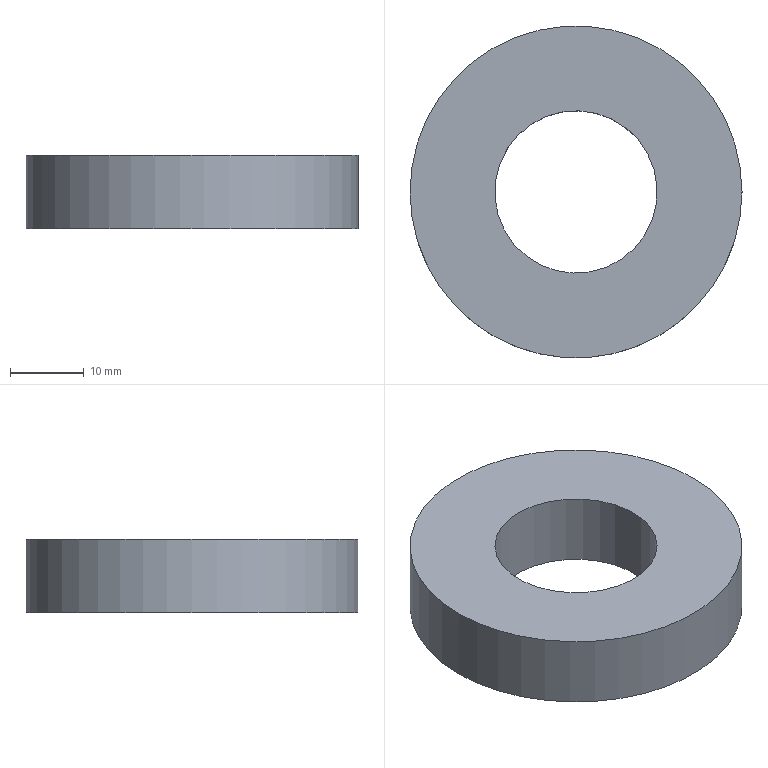Part | NX | features solid 2 | 1 solid | 4 faces | box 45 x 45 x 10 mm | volume 12103 mm3 | cylinder 2 | plane 2 | commonest cylinder face diameters 22 x1 45 x1
STEP:
#1=CARTESIAN_POINT('',(644.963,510.927,170.));
#2=VERTEX_POINT('',#1);
#3=CARTESIAN_POINT('',(643.053,521.759,170.));
#4=DIRECTION('',(0.,0.,1.));
#5=DIRECTION('',(0.1736,-0.9848,0.));
#6=AXIS2_PLACEMENT_3D('',#3,#4,#5);
#7=CIRCLE('',#6,11.);
#8=EDGE_CURVE('',#2,#2,#7,.T.);
#9=ORIENTED_EDGE('',*,*,#8,.F.);
#10=EDGE_LOOP('',(#9));
#11=FACE_BOUND('',#10,.T.);
#12=CARTESIAN_POINT('',(644.963,510.927,180.));
#13=VERTEX_POINT('',#12);
#14=CARTESIAN_POINT('',(643.053,521.759,180.));
#15=DIRECTION('',(0.,0.,1.));
#16=DIRECTION('',(0.1736,-0.9848,0.));
#17=AXIS2_PLACEMENT_3D('',#14,#15,#16);
#18=CIRCLE('',#17,11.);
#19=EDGE_CURVE('',#13,#13,#18,.T.);
#20=ORIENTED_EDGE('',*,*,#19,.T.);
#21=EDGE_LOOP('',(#20));
#22=FACE_BOUND('',#21,.T.);
#23=CARTESIAN_POINT('',(643.053,521.759,170.));
#24=DIRECTION('',(0.,0.,1.));
#25=DIRECTION('',(0.1736,-0.9848,0.));
#26=AXIS2_PLACEMENT_3D('',#23,#24,#25);
#27=CYLINDRICAL_SURFACE('',#26,11.);
#28=ADVANCED_FACE('',(#11,#22),#27,.F.);
#29=CARTESIAN_POINT('',(665.553,521.759,170.));
#30=VERTEX_POINT('',#29);
#31=CARTESIAN_POINT('',(643.053,521.759,170.));
#32=DIRECTION('',(0.,0.,1.));
#33=DIRECTION('',(1.,0.,0.));
#34=AXIS2_PLACEMENT_3D('',#31,#32,#33);
#35=CIRCLE('',#34,22.5);
#36=EDGE_CURVE('',#30,#30,#35,.T.);
#37=ORIENTED_EDGE('',*,*,#36,.T.);
#38=EDGE_LOOP('',(#37));
#39=FACE_BOUND('',#38,.T.);
#40=CARTESIAN_POINT('',(665.553,521.759,180.));
#41=VERTEX_POINT('',#40);
#42=CARTESIAN_POINT('',(643.053,521.759,180.));
#43=DIRECTION('',(0.,0.,1.));
#44=DIRECTION('',(1.,0.,0.));
#45=AXIS2_PLACEMENT_3D('',#42,#43,#44);
#46=CIRCLE('',#45,22.5);
#47=EDGE_CURVE('',#41,#41,#46,.T.);
#48=ORIENTED_EDGE('',*,*,#47,.F.);
#49=EDGE_LOOP('',(#48));
#50=FACE_BOUND('',#49,.T.);
#51=CARTESIAN_POINT('',(643.053,521.759,170.));
#52=DIRECTION('',(0.,0.,1.));
#53=DIRECTION('',(0.1736,-0.9848,0.));
#54=AXIS2_PLACEMENT_3D('',#51,#52,#53);
#55=CYLINDRICAL_SURFACE('',#54,22.5);
#56=ADVANCED_FACE('',(#39,#50),#55,.T.);
#57=ORIENTED_EDGE('',*,*,#8,.T.);
#58=EDGE_LOOP('',(#57));
#59=FACE_BOUND('',#58,.T.);
#60=ORIENTED_EDGE('',*,*,#36,.F.);
#61=EDGE_LOOP('',(#60));
#62=FACE_BOUND('',#61,.T.);
#63=CARTESIAN_POINT('',(643.053,521.759,170.));
#64=DIRECTION('',(0.,0.,1.));
#65=DIRECTION('',(-0.1736,0.9848,0.));
#66=AXIS2_PLACEMENT_3D('',#63,#64,#65);
#67=PLANE('',#66);
#68=ADVANCED_FACE('',(#59,#62),#67,.F.);
#69=ORIENTED_EDGE('',*,*,#19,.F.);
#70=EDGE_LOOP('',(#69));
#71=FACE_BOUND('',#70,.T.);
#72=ORIENTED_EDGE('',*,*,#47,.T.);
#73=EDGE_LOOP('',(#72));
#74=FACE_BOUND('',#73,.T.);
#75=CARTESIAN_POINT('',(643.053,521.759,180.));
#76=DIRECTION('',(0.,0.,1.));
#77=DIRECTION('',(-0.1736,0.9848,0.));
#78=AXIS2_PLACEMENT_3D('',#75,#76,#77);
#79=PLANE('',#78);
#80=ADVANCED_FACE('',(#71,#74),#79,.T.);
#81=CLOSED_SHELL('',(#28,#56,#68,#80));
#82=MANIFOLD_SOLID_BREP('',#81);
#83=(LENGTH_UNIT()NAMED_UNIT(*)SI_UNIT(.MILLI.,.METRE.));
#84=UNCERTAINTY_MEASURE_WITH_UNIT(LENGTH_MEASURE(0.00001),#83,'','');
#85=(NAMED_UNIT(*)PLANE_ANGLE_UNIT()SI_UNIT($,.RADIAN.));
#86=(NAMED_UNIT(*)SI_UNIT($,.STERADIAN.)SOLID_ANGLE_UNIT());
#87=(GEOMETRIC_REPRESENTATION_CONTEXT(3)GLOBAL_UNCERTAINTY_ASSIGNED_CONTEXT((#84))GLOBAL_UNIT_ASSIGNED_CONTEXT((#83,#85,#86))REPRESENTATION_CONTEXT('',''));
#88=ADVANCED_BREP_SHAPE_REPRESENTATION('',(#82),#87);